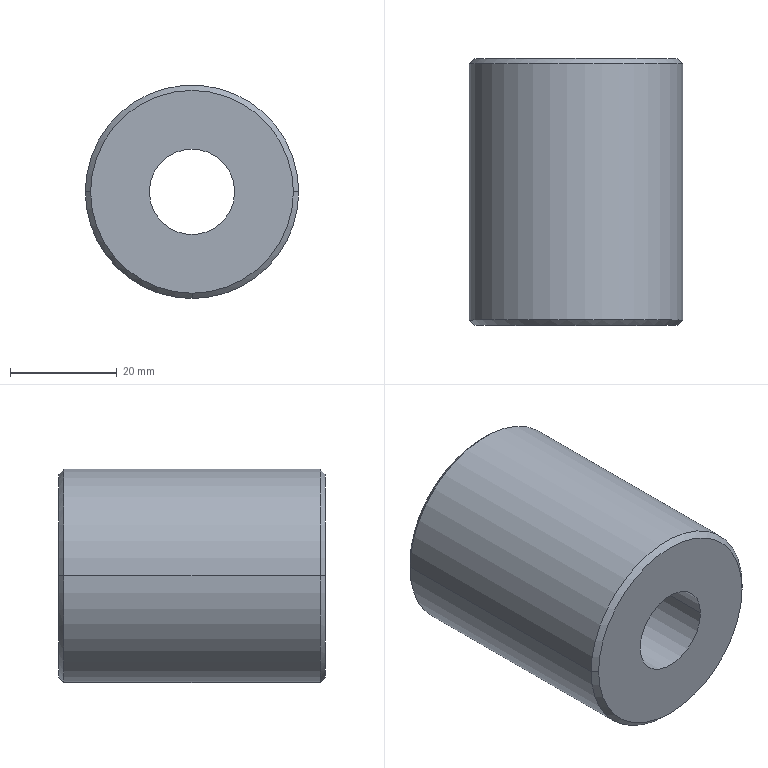Part | NX | features BREP 1 | 1 solid | 15 faces | box 40 x 50 x 40 mm | volume 51320 mm3 | cylinder 6 | cone 6 | plane 3 | commonest cylinder face diameters 16 x2 18 x2 40 x2
STEP:
#1=CARTESIAN_POINT('',(-19.,0.,0.));
#2=VERTEX_POINT('',#1);
#3=CARTESIAN_POINT('',(0.,0.,-19.));
#4=VERTEX_POINT('',#3);
#5=CARTESIAN_POINT('',(0.,0.,0.));
#6=DIRECTION('',(0.,-1.,0.));
#7=DIRECTION('',(-1.,0.,0.));
#8=AXIS2_PLACEMENT_3D('',#5,#6,#7);
#9=CIRCLE('',#8,19.);
#10=EDGE_CURVE('',#2,#4,#9,.T.);
#11=ORIENTED_EDGE('',*,*,#10,.T.);
#12=CARTESIAN_POINT('',(19.,0.,0.));
#13=VERTEX_POINT('',#12);
#14=CARTESIAN_POINT('',(0.,0.,0.));
#15=DIRECTION('',(0.,-1.,0.));
#16=DIRECTION('',(-1.,0.,0.));
#17=AXIS2_PLACEMENT_3D('',#14,#15,#16);
#18=CIRCLE('',#17,19.);
#19=EDGE_CURVE('',#4,#13,#18,.T.);
#20=ORIENTED_EDGE('',*,*,#19,.T.);
#21=CARTESIAN_POINT('',(0.,0.,0.));
#22=DIRECTION('',(0.,-1.,0.));
#23=DIRECTION('',(1.,0.,0.));
#24=AXIS2_PLACEMENT_3D('',#21,#22,#23);
#25=CIRCLE('',#24,19.);
#26=EDGE_CURVE('',#13,#2,#25,.T.);
#27=ORIENTED_EDGE('',*,*,#26,.T.);
#28=EDGE_LOOP('',(#11,#20,#27));
#29=FACE_BOUND('',#28,.T.);
#30=CARTESIAN_POINT('',(8.,0.,0.));
#31=VERTEX_POINT('',#30);
#32=CARTESIAN_POINT('',(-8.,0.,0.));
#33=VERTEX_POINT('',#32);
#34=CARTESIAN_POINT('',(0.,0.,0.));
#35=DIRECTION('',(0.,-1.,0.));
#36=DIRECTION('',(1.,0.,0.));
#37=AXIS2_PLACEMENT_3D('',#34,#35,#36);
#38=CIRCLE('',#37,8.);
#39=EDGE_CURVE('',#31,#33,#38,.T.);
#40=ORIENTED_EDGE('',*,*,#39,.F.);
#41=CARTESIAN_POINT('',(0.,0.,0.));
#42=DIRECTION('',(0.,-1.,0.));
#43=DIRECTION('',(-1.,0.,0.));
#44=AXIS2_PLACEMENT_3D('',#41,#42,#43);
#45=CIRCLE('',#44,8.);
#46=EDGE_CURVE('',#33,#31,#45,.T.);
#47=ORIENTED_EDGE('',*,*,#46,.F.);
#48=EDGE_LOOP('',(#40,#47));
#49=FACE_BOUND('',#48,.T.);
#50=CARTESIAN_POINT('',(0.,0.,0.));
#51=DIRECTION('',(0.,1.,0.));
#52=DIRECTION('',(1.,0.,0.));
#53=AXIS2_PLACEMENT_3D('',#50,#51,#52);
#54=PLANE('',#53);
#55=ADVANCED_FACE('',(#29,#49),#54,.F.);
#56=CARTESIAN_POINT('',(8.,25.,0.));
#57=VERTEX_POINT('',#56);
#58=CARTESIAN_POINT('',(8.,0.,0.));
#59=DIRECTION('',(0.,1.,0.));
#60=VECTOR('',#59,1000.);
#61=LINE('',#58,#60);
#62=EDGE_CURVE('',#57,#31,#61,.F.);
#63=ORIENTED_EDGE('',*,*,#62,.F.);
#64=CARTESIAN_POINT('',(-8.,25.,0.));
#65=VERTEX_POINT('',#64);
#66=CARTESIAN_POINT('',(0.,25.,0.));
#67=DIRECTION('',(0.,-1.,0.));
#68=DIRECTION('',(-1.,0.,0.));
#69=AXIS2_PLACEMENT_3D('',#66,#67,#68);
#70=CIRCLE('',#69,8.);
#71=EDGE_CURVE('',#65,#57,#70,.T.);
#72=ORIENTED_EDGE('',*,*,#71,.F.);
#73=CARTESIAN_POINT('',(-8.,0.,0.));
#74=DIRECTION('',(0.,1.,0.));
#75=VECTOR('',#74,1000.);
#76=LINE('',#73,#75);
#77=EDGE_CURVE('',#65,#33,#76,.F.);
#78=ORIENTED_EDGE('',*,*,#77,.T.);
#79=ORIENTED_EDGE('',*,*,#46,.T.);
#80=EDGE_LOOP('',(#63,#72,#78,#79));
#81=FACE_BOUND('',#80,.T.);
#82=CARTESIAN_POINT('',(0.,0.,0.));
#83=DIRECTION('',(0.,-1.,0.));
#84=DIRECTION('',(-1.,0.,0.));
#85=AXIS2_PLACEMENT_3D('',#82,#83,#84);
#86=CYLINDRICAL_SURFACE('',#85,8.);
#87=ADVANCED_FACE('',(#81),#86,.F.);
#88=ORIENTED_EDGE('',*,*,#77,.F.);
#89=CARTESIAN_POINT('',(0.,25.,0.));
#90=DIRECTION('',(0.,-1.,0.));
#91=DIRECTION('',(1.,0.,0.));
#92=AXIS2_PLACEMENT_3D('',#89,#90,#91);
#93=CIRCLE('',#92,8.);
#94=EDGE_CURVE('',#57,#65,#93,.T.);
#95=ORIENTED_EDGE('',*,*,#94,.F.);
#96=ORIENTED_EDGE('',*,*,#62,.T.);
#97=ORIENTED_EDGE('',*,*,#39,.T.);
#98=EDGE_LOOP('',(#88,#95,#96,#97));
#99=FACE_BOUND('',#98,.T.);
#100=CARTESIAN_POINT('',(0.,0.,0.));
#101=DIRECTION('',(0.,-1.,0.));
#102=DIRECTION('',(-1.,0.,0.));
#103=AXIS2_PLACEMENT_3D('',#100,#101,#102);
#104=CYLINDRICAL_SURFACE('',#103,8.);
#105=ADVANCED_FACE('',(#99),#104,.F.);
#106=CARTESIAN_POINT('',(-9.,25.,0.));
#107=VERTEX_POINT('',#106);
#108=CARTESIAN_POINT('',(9.,25.,0.));
#109=VERTEX_POINT('',#108);
#110=CARTESIAN_POINT('',(0.,25.,0.));
#111=DIRECTION('',(0.,1.,0.));
#112=DIRECTION('',(-1.,0.,0.));
#113=AXIS2_PLACEMENT_3D('',#110,#111,#112);
#114=CIRCLE('',#113,9.);
#115=EDGE_CURVE('',#107,#109,#114,.T.);
#116=ORIENTED_EDGE('',*,*,#115,.T.);
#117=CARTESIAN_POINT('',(0.,25.,0.));
#118=DIRECTION('',(0.,1.,0.));
#119=DIRECTION('',(1.,0.,0.));
#120=AXIS2_PLACEMENT_3D('',#117,#118,#119);
#121=CIRCLE('',#120,9.);
#122=EDGE_CURVE('',#109,#107,#121,.T.);
#123=ORIENTED_EDGE('',*,*,#122,.T.);
#124=EDGE_LOOP('',(#116,#123));
#125=FACE_BOUND('',#124,.T.);
#126=ORIENTED_EDGE('',*,*,#94,.T.);
#127=ORIENTED_EDGE('',*,*,#71,.T.);
#128=EDGE_LOOP('',(#126,#127));
#129=FACE_BOUND('',#128,.T.);
#130=CARTESIAN_POINT('',(0.,25.,0.));
#131=DIRECTION('',(0.,1.,0.));
#132=DIRECTION('',(1.,0.,0.));
#133=AXIS2_PLACEMENT_3D('',#130,#131,#132);
#134=PLANE('',#133);
#135=ADVANCED_FACE('',(#125,#129),#134,.T.);
#136=CARTESIAN_POINT('',(-9.,50.,0.));
#137=VERTEX_POINT('',#136);
#138=CARTESIAN_POINT('',(-9.,50.,0.));
#139=DIRECTION('',(0.,-1.,0.));
#140=VECTOR('',#139,1000.);
#141=LINE('',#138,#140);
#142=EDGE_CURVE('',#137,#107,#141,.T.);
#143=ORIENTED_EDGE('',*,*,#142,.T.);
#144=ORIENTED_EDGE('',*,*,#122,.F.);
#145=CARTESIAN_POINT('',(9.,50.,0.));
#146=VERTEX_POINT('',#145);
#147=CARTESIAN_POINT('',(9.,50.,0.));
#148=DIRECTION('',(0.,-1.,0.));
#149=VECTOR('',#148,1000.);
#150=LINE('',#147,#149);
#151=EDGE_CURVE('',#146,#109,#150,.T.);
#152=ORIENTED_EDGE('',*,*,#151,.F.);
#153=CARTESIAN_POINT('',(0.,50.,0.));
#154=DIRECTION('',(0.,1.,0.));
#155=DIRECTION('',(1.,0.,0.));
#156=AXIS2_PLACEMENT_3D('',#153,#154,#155);
#157=CIRCLE('',#156,9.);
#158=EDGE_CURVE('',#146,#137,#157,.T.);
#159=ORIENTED_EDGE('',*,*,#158,.T.);
#160=EDGE_LOOP('',(#143,#144,#152,#159));
#161=FACE_BOUND('',#160,.T.);
#162=CARTESIAN_POINT('',(0.,50.,0.));
#163=DIRECTION('',(0.,1.,0.));
#164=DIRECTION('',(1.,0.,0.));
#165=AXIS2_PLACEMENT_3D('',#162,#163,#164);
#166=CYLINDRICAL_SURFACE('',#165,9.);
#167=ADVANCED_FACE('',(#161),#166,.F.);
#168=CARTESIAN_POINT('',(19.,50.,0.));
#169=VERTEX_POINT('',#168);
#170=CARTESIAN_POINT('',(0.,50.,-19.));
#171=VERTEX_POINT('',#170);
#172=CARTESIAN_POINT('',(0.,50.,0.));
#173=DIRECTION('',(0.,1.,0.));
#174=DIRECTION('',(1.,0.,0.));
#175=AXIS2_PLACEMENT_3D('',#172,#173,#174);
#176=CIRCLE('',#175,19.);
#177=EDGE_CURVE('',#169,#171,#176,.T.);
#178=ORIENTED_EDGE('',*,*,#177,.T.);
#179=CARTESIAN_POINT('',(-19.,50.,0.));
#180=VERTEX_POINT('',#179);
#181=CARTESIAN_POINT('',(0.,50.,0.));
#182=DIRECTION('',(0.,1.,0.));
#183=DIRECTION('',(1.,0.,0.));
#184=AXIS2_PLACEMENT_3D('',#181,#182,#183);
#185=CIRCLE('',#184,19.);
#186=EDGE_CURVE('',#171,#180,#185,.T.);
#187=ORIENTED_EDGE('',*,*,#186,.T.);
#188=CARTESIAN_POINT('',(0.,50.,0.));
#189=DIRECTION('',(0.,1.,0.));
#190=DIRECTION('',(-1.,0.,0.));
#191=AXIS2_PLACEMENT_3D('',#188,#189,#190);
#192=CIRCLE('',#191,19.);
#193=EDGE_CURVE('',#180,#169,#192,.T.);
#194=ORIENTED_EDGE('',*,*,#193,.T.);
#195=EDGE_LOOP('',(#178,#187,#194));
#196=FACE_BOUND('',#195,.T.);
#197=CARTESIAN_POINT('',(0.,50.,0.));
#198=DIRECTION('',(0.,1.,0.));
#199=DIRECTION('',(-1.,0.,0.));
#200=AXIS2_PLACEMENT_3D('',#197,#198,#199);
#201=CIRCLE('',#200,9.);
#202=EDGE_CURVE('',#137,#146,#201,.T.);
#203=ORIENTED_EDGE('',*,*,#202,.F.);
#204=ORIENTED_EDGE('',*,*,#158,.F.);
#205=EDGE_LOOP('',(#203,#204));
#206=FACE_BOUND('',#205,.T.);
#207=CARTESIAN_POINT('',(0.,50.,0.));
#208=DIRECTION('',(0.,1.,0.));
#209=DIRECTION('',(1.,0.,0.));
#210=AXIS2_PLACEMENT_3D('',#207,#208,#209);
#211=PLANE('',#210);
#212=ADVANCED_FACE('',(#196,#206),#211,.T.);
#213=ORIENTED_EDGE('',*,*,#151,.T.);
#214=ORIENTED_EDGE('',*,*,#115,.F.);
#215=ORIENTED_EDGE('',*,*,#142,.F.);
#216=ORIENTED_EDGE('',*,*,#202,.T.);
#217=EDGE_LOOP('',(#213,#214,#215,#216));
#218=FACE_BOUND('',#217,.T.);
#219=CARTESIAN_POINT('',(0.,50.,0.));
#220=DIRECTION('',(0.,1.,0.));
#221=DIRECTION('',(1.,0.,0.));
#222=AXIS2_PLACEMENT_3D('',#219,#220,#221);
#223=CYLINDRICAL_SURFACE('',#222,9.);
#224=ADVANCED_FACE('',(#218),#223,.F.);
#225=CARTESIAN_POINT('',(-20.,49.,0.));
#226=VERTEX_POINT('',#225);
#227=CARTESIAN_POINT('',(-19.,50.,0.000000003));
#228=DIRECTION('',(-0.7071,-0.7071,0.));
#229=VECTOR('',#228,1000.);
#230=LINE('',#227,#229);
#231=EDGE_CURVE('',#180,#226,#230,.T.);
#232=ORIENTED_EDGE('',*,*,#231,.T.);
#233=CARTESIAN_POINT('',(20.,49.,0.));
#234=VERTEX_POINT('',#233);
#235=CARTESIAN_POINT('',(0.,49.,0.));
#236=DIRECTION('',(0.,1.,0.));
#237=DIRECTION('',(-1.,0.,0.));
#238=AXIS2_PLACEMENT_3D('',#235,#236,#237);
#239=CIRCLE('',#238,20.);
#240=EDGE_CURVE('',#226,#234,#239,.T.);
#241=ORIENTED_EDGE('',*,*,#240,.T.);
#242=CARTESIAN_POINT('',(19.,50.,-0.000000003));
#243=DIRECTION('',(0.7071,-0.7071,0.));
#244=VECTOR('',#243,1000.);
#245=LINE('',#242,#244);
#246=EDGE_CURVE('',#169,#234,#245,.T.);
#247=ORIENTED_EDGE('',*,*,#246,.F.);
#248=ORIENTED_EDGE('',*,*,#193,.F.);
#249=EDGE_LOOP('',(#232,#241,#247,#248));
#250=FACE_BOUND('',#249,.T.);
#251=CARTESIAN_POINT('',(0.,49.5,0.));
#252=DIRECTION('',(0.,-1.,0.));
#253=DIRECTION('',(0.,0.,-1.));
#254=AXIS2_PLACEMENT_3D('',#251,#252,#253);
#255=CONICAL_SURFACE('',#254,19.5,0.7854);
#256=ADVANCED_FACE('',(#250),#255,.T.);
#257=CARTESIAN_POINT('',(0.,49.,-20.));
#258=VERTEX_POINT('',#257);
#259=CARTESIAN_POINT('',(0.,49.5,-19.5));
#260=DIRECTION('',(0.,-0.7071,-0.7071));
#261=VECTOR('',#260,1000.);
#262=LINE('',#259,#261);
#263=EDGE_CURVE('',#171,#258,#262,.T.);
#264=ORIENTED_EDGE('',*,*,#263,.F.);
#265=ORIENTED_EDGE('',*,*,#177,.F.);
#266=ORIENTED_EDGE('',*,*,#246,.T.);
#267=CARTESIAN_POINT('',(0.,49.,0.));
#268=DIRECTION('',(0.,1.,0.));
#269=DIRECTION('',(1.,0.,0.));
#270=AXIS2_PLACEMENT_3D('',#267,#268,#269);
#271=CIRCLE('',#270,20.);
#272=EDGE_CURVE('',#234,#258,#271,.T.);
#273=ORIENTED_EDGE('',*,*,#272,.T.);
#274=EDGE_LOOP('',(#264,#265,#266,#273));
#275=FACE_BOUND('',#274,.T.);
#276=CARTESIAN_POINT('',(0.,49.5,0.));
#277=DIRECTION('',(0.,-1.,0.));
#278=DIRECTION('',(0.,0.,-1.));
#279=AXIS2_PLACEMENT_3D('',#276,#277,#278);
#280=CONICAL_SURFACE('',#279,19.5,0.7854);
#281=ADVANCED_FACE('',(#275),#280,.T.);
#282=CARTESIAN_POINT('',(20.,1.,0.));
#283=VERTEX_POINT('',#282);
#284=CARTESIAN_POINT('',(20.,1.,-0.000000003));
#285=DIRECTION('',(0.,1.,0.));
#286=VECTOR('',#285,1000.);
#287=LINE('',#284,#286);
#288=EDGE_CURVE('',#234,#283,#287,.F.);
#289=ORIENTED_EDGE('',*,*,#288,.T.);
#290=CARTESIAN_POINT('',(0.,1.,-20.));
#291=VERTEX_POINT('',#290);
#292=CARTESIAN_POINT('',(0.,1.,0.));
#293=DIRECTION('',(0.,-1.,0.));
#294=DIRECTION('',(-1.,0.,0.));
#295=AXIS2_PLACEMENT_3D('',#292,#293,#294);
#296=CIRCLE('',#295,20.);
#297=EDGE_CURVE('',#291,#283,#296,.T.);
#298=ORIENTED_EDGE('',*,*,#297,.F.);
#299=CARTESIAN_POINT('',(-20.,1.,0.));
#300=VERTEX_POINT('',#299);
#301=CARTESIAN_POINT('',(0.,1.,0.));
#302=DIRECTION('',(0.,-1.,0.));
#303=DIRECTION('',(-1.,0.,0.));
#304=AXIS2_PLACEMENT_3D('',#301,#302,#303);
#305=CIRCLE('',#304,20.);
#306=EDGE_CURVE('',#300,#291,#305,.T.);
#307=ORIENTED_EDGE('',*,*,#306,.F.);
#308=CARTESIAN_POINT('',(-20.,1.,0.000000003));
#309=DIRECTION('',(0.,1.,0.));
#310=VECTOR('',#309,1000.);
#311=LINE('',#308,#310);
#312=EDGE_CURVE('',#226,#300,#311,.F.);
#313=ORIENTED_EDGE('',*,*,#312,.F.);
#314=CARTESIAN_POINT('',(0.,49.,0.));
#315=DIRECTION('',(0.,1.,0.));
#316=DIRECTION('',(1.,0.,0.));
#317=AXIS2_PLACEMENT_3D('',#314,#315,#316);
#318=CIRCLE('',#317,20.);
#319=EDGE_CURVE('',#258,#226,#318,.T.);
#320=ORIENTED_EDGE('',*,*,#319,.F.);
#321=ORIENTED_EDGE('',*,*,#272,.F.);
#322=EDGE_LOOP('',(#289,#298,#307,#313,#320,#321));
#323=FACE_BOUND('',#322,.T.);
#324=CARTESIAN_POINT('',(0.,0.,0.));
#325=DIRECTION('',(0.,1.,0.));
#326=DIRECTION('',(1.,0.,0.));
#327=AXIS2_PLACEMENT_3D('',#324,#325,#326);
#328=CYLINDRICAL_SURFACE('',#327,20.);
#329=ADVANCED_FACE('',(#323),#328,.T.);
#330=ORIENTED_EDGE('',*,*,#312,.T.);
#331=CARTESIAN_POINT('',(0.,1.,0.));
#332=DIRECTION('',(0.,-1.,0.));
#333=DIRECTION('',(1.,0.,0.));
#334=AXIS2_PLACEMENT_3D('',#331,#332,#333);
#335=CIRCLE('',#334,20.);
#336=EDGE_CURVE('',#283,#300,#335,.T.);
#337=ORIENTED_EDGE('',*,*,#336,.F.);
#338=ORIENTED_EDGE('',*,*,#288,.F.);
#339=ORIENTED_EDGE('',*,*,#240,.F.);
#340=EDGE_LOOP('',(#330,#337,#338,#339));
#341=FACE_BOUND('',#340,.T.);
#342=CARTESIAN_POINT('',(0.,0.,0.));
#343=DIRECTION('',(0.,1.,0.));
#344=DIRECTION('',(1.,0.,0.));
#345=AXIS2_PLACEMENT_3D('',#342,#343,#344);
#346=CYLINDRICAL_SURFACE('',#345,20.);
#347=ADVANCED_FACE('',(#341),#346,.T.);
#348=CARTESIAN_POINT('',(19.,0.,-0.000000003));
#349=DIRECTION('',(0.7071,0.7071,0.));
#350=VECTOR('',#349,1000.);
#351=LINE('',#348,#350);
#352=EDGE_CURVE('',#13,#283,#351,.T.);
#353=ORIENTED_EDGE('',*,*,#352,.T.);
#354=ORIENTED_EDGE('',*,*,#336,.T.);
#355=CARTESIAN_POINT('',(-19.,0.,0.000000003));
#356=DIRECTION('',(-0.7071,0.7071,0.));
#357=VECTOR('',#356,1000.);
#358=LINE('',#355,#357);
#359=EDGE_CURVE('',#2,#300,#358,.T.);
#360=ORIENTED_EDGE('',*,*,#359,.F.);
#361=ORIENTED_EDGE('',*,*,#26,.F.);
#362=EDGE_LOOP('',(#353,#354,#360,#361));
#363=FACE_BOUND('',#362,.T.);
#364=CARTESIAN_POINT('',(0.,0.5,0.));
#365=DIRECTION('',(0.,1.,0.));
#366=DIRECTION('',(0.,0.,-1.));
#367=AXIS2_PLACEMENT_3D('',#364,#365,#366);
#368=CONICAL_SURFACE('',#367,19.5,0.7854);
#369=ADVANCED_FACE('',(#363),#368,.T.);
#370=CARTESIAN_POINT('',(0.,0.5,-19.5));
#371=DIRECTION('',(0.,0.7071,-0.7071));
#372=VECTOR('',#371,1000.);
#373=LINE('',#370,#372);
#374=EDGE_CURVE('',#4,#291,#373,.T.);
#375=ORIENTED_EDGE('',*,*,#374,.F.);
#376=ORIENTED_EDGE('',*,*,#10,.F.);
#377=ORIENTED_EDGE('',*,*,#359,.T.);
#378=ORIENTED_EDGE('',*,*,#306,.T.);
#379=EDGE_LOOP('',(#375,#376,#377,#378));
#380=FACE_BOUND('',#379,.T.);
#381=CARTESIAN_POINT('',(0.,0.5,0.));
#382=DIRECTION('',(0.,1.,0.));
#383=DIRECTION('',(0.,0.,-1.));
#384=AXIS2_PLACEMENT_3D('',#381,#382,#383);
#385=CONICAL_SURFACE('',#384,19.5,0.7854);
#386=ADVANCED_FACE('',(#380),#385,.T.);
#387=ORIENTED_EDGE('',*,*,#19,.F.);
#388=ORIENTED_EDGE('',*,*,#374,.T.);
#389=ORIENTED_EDGE('',*,*,#297,.T.);
#390=ORIENTED_EDGE('',*,*,#352,.F.);
#391=EDGE_LOOP('',(#387,#388,#389,#390));
#392=FACE_BOUND('',#391,.T.);
#393=CARTESIAN_POINT('',(0.,0.5,0.));
#394=DIRECTION('',(0.,1.,0.));
#395=DIRECTION('',(0.,0.,-1.));
#396=AXIS2_PLACEMENT_3D('',#393,#394,#395);
#397=CONICAL_SURFACE('',#396,19.5,0.7854);
#398=ADVANCED_FACE('',(#392),#397,.T.);
#399=ORIENTED_EDGE('',*,*,#186,.F.);
#400=ORIENTED_EDGE('',*,*,#263,.T.);
#401=ORIENTED_EDGE('',*,*,#319,.T.);
#402=ORIENTED_EDGE('',*,*,#231,.F.);
#403=EDGE_LOOP('',(#399,#400,#401,#402));
#404=FACE_BOUND('',#403,.T.);
#405=CARTESIAN_POINT('',(0.,49.5,0.));
#406=DIRECTION('',(0.,-1.,0.));
#407=DIRECTION('',(0.,0.,-1.));
#408=AXIS2_PLACEMENT_3D('',#405,#406,#407);
#409=CONICAL_SURFACE('',#408,19.5,0.7854);
#410=ADVANCED_FACE('',(#404),#409,.T.);
#411=CLOSED_SHELL('',(#55,#87,#105,#135,#167,#212,#224,#256,#281,#329,#347,#369,#386,#398,#410));
#412=MANIFOLD_SOLID_BREP('',#411);
#413=(LENGTH_UNIT()NAMED_UNIT(*)SI_UNIT(.MILLI.,.METRE.));
#414=UNCERTAINTY_MEASURE_WITH_UNIT(LENGTH_MEASURE(0.00001),#413,'','');
#415=(NAMED_UNIT(*)PLANE_ANGLE_UNIT()SI_UNIT($,.RADIAN.));
#416=(NAMED_UNIT(*)SI_UNIT($,.STERADIAN.)SOLID_ANGLE_UNIT());
#417=(GEOMETRIC_REPRESENTATION_CONTEXT(3)GLOBAL_UNCERTAINTY_ASSIGNED_CONTEXT((#414))GLOBAL_UNIT_ASSIGNED_CONTEXT((#413,#415,#416))REPRESENTATION_CONTEXT('',''));
#418=ADVANCED_BREP_SHAPE_REPRESENTATION('',(#412),#417);